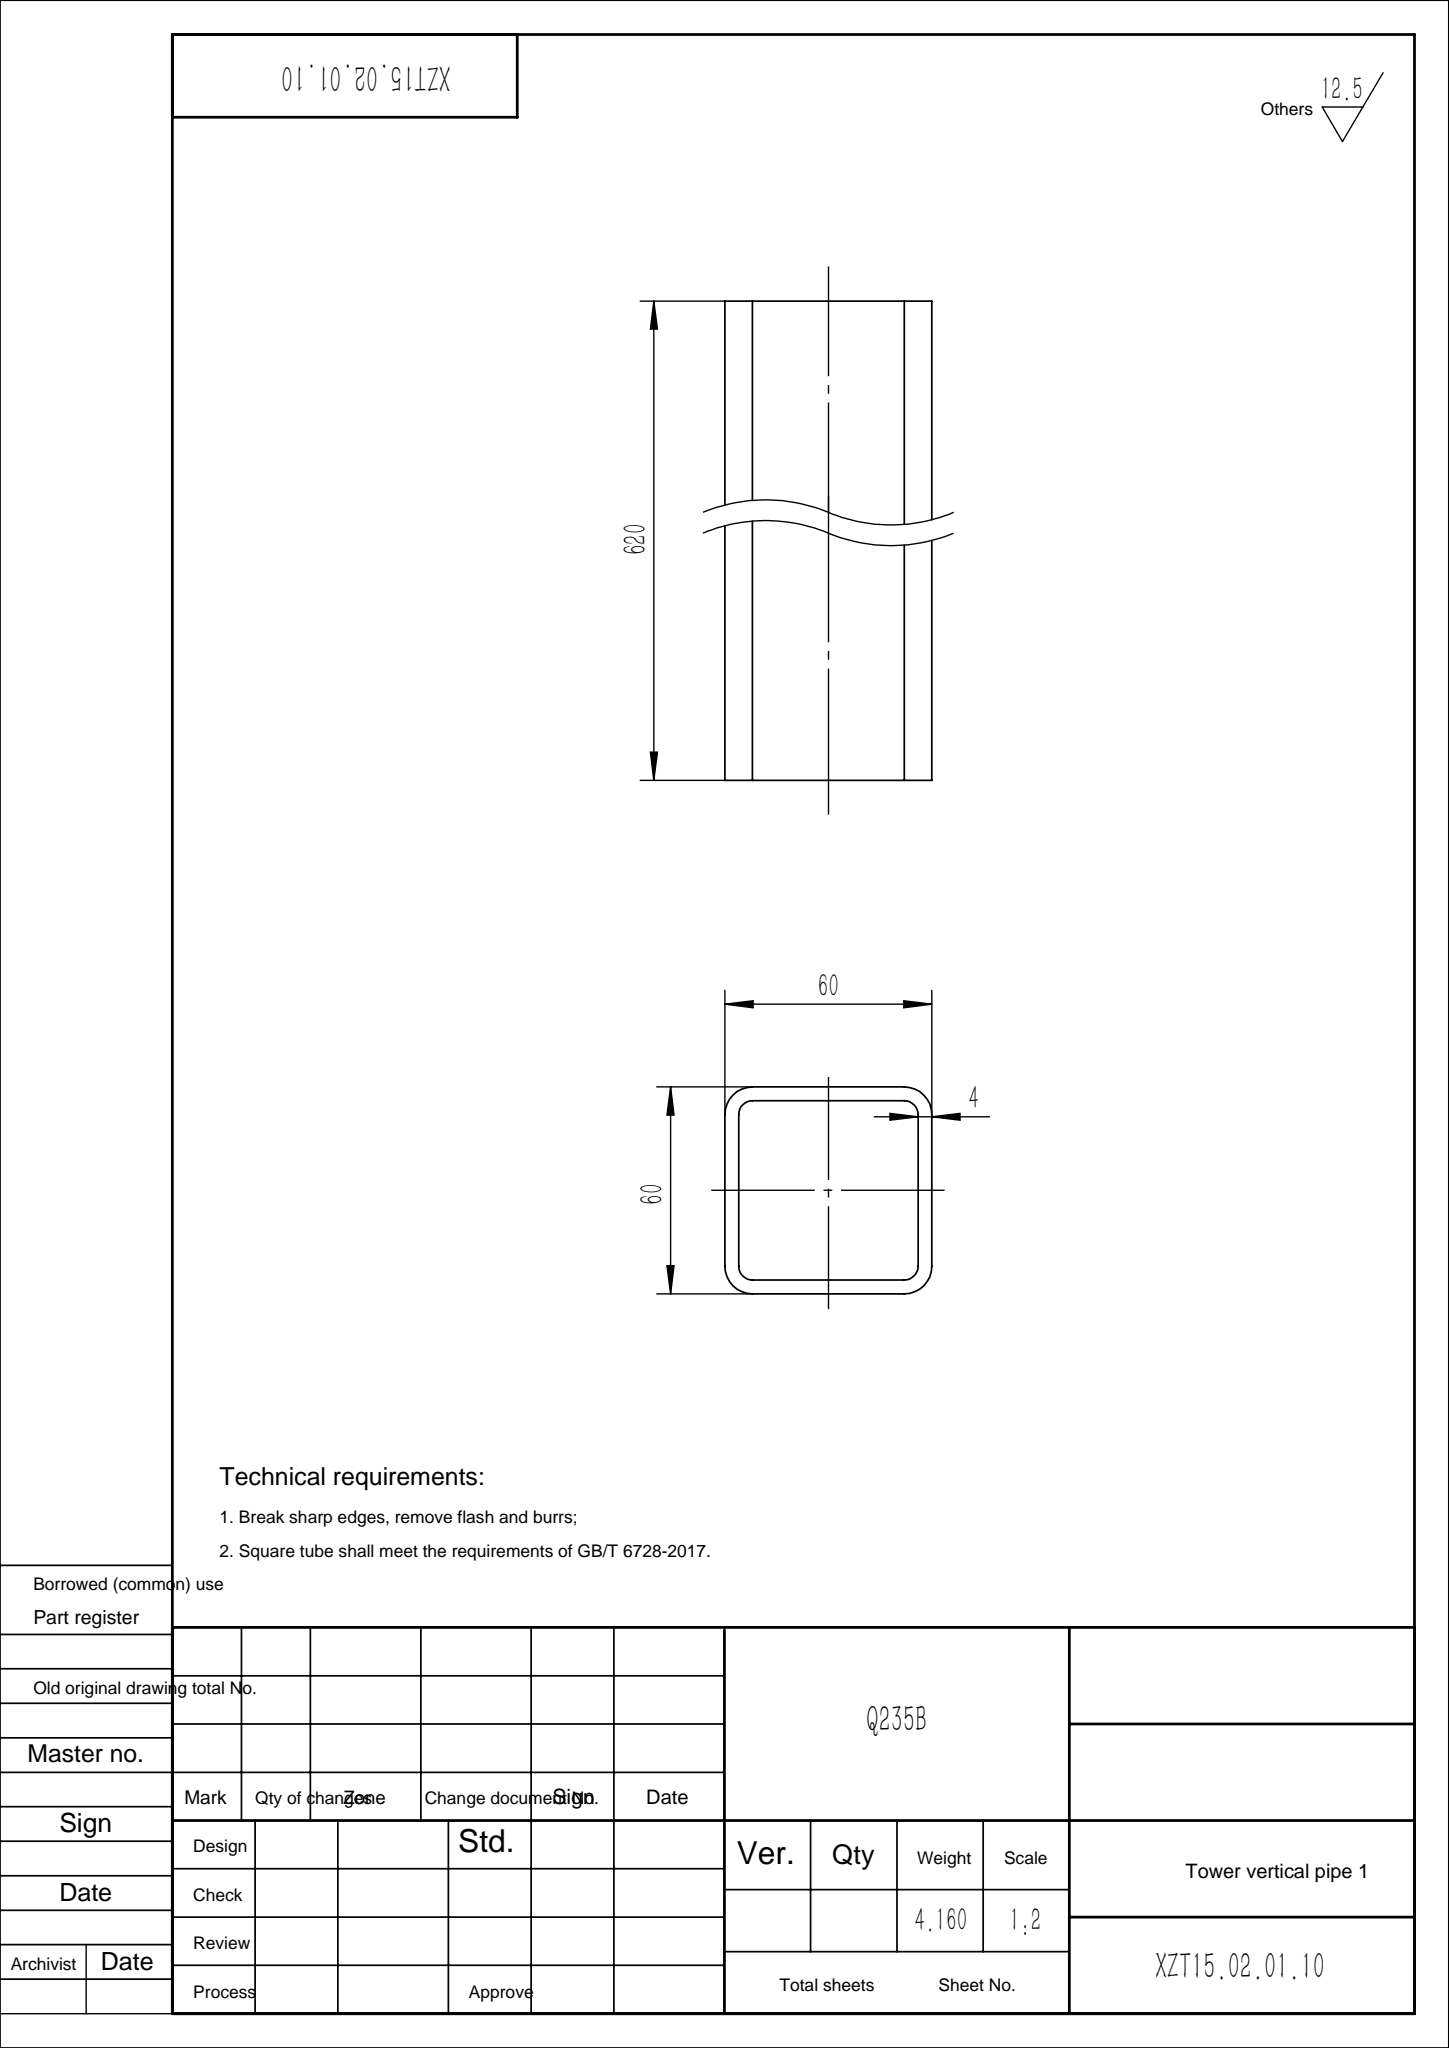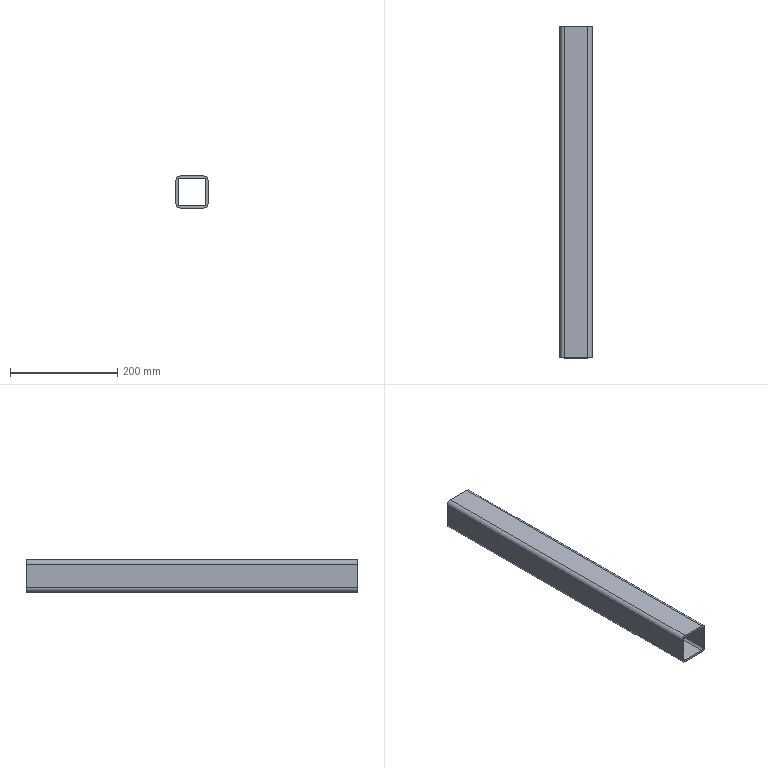Part | SolidWorks | features WeldMemberFeat 1, WeldmentFeature 1 | 1 solid | 18 faces | box 60 x 620 x 60 mm | volume 529974 mm3 | plane 10 | cylinder 8 | commonest cylinder face diameters 8 x4 16 x4
STEP:
#1=CARTESIAN_POINT('',(-30.,0.,22.));
#2=VERTEX_POINT('',#1);
#3=CARTESIAN_POINT('',(-22.,0.,30.));
#4=VERTEX_POINT('',#3);
#5=CARTESIAN_POINT('',(-22.,0.,22.));
#6=DIRECTION('',(0.,1.,0.));
#7=DIRECTION('',(0.,0.,1.));
#8=AXIS2_PLACEMENT_3D('',#5,#6,#7);
#9=CIRCLE('',#8,8.);
#10=EDGE_CURVE('',#2,#4,#9,.T.);
#11=ORIENTED_EDGE('',*,*,#10,.T.);
#12=CARTESIAN_POINT('',(-22.,620.,30.));
#13=VERTEX_POINT('',#12);
#14=CARTESIAN_POINT('',(-22.,620.,30.));
#15=DIRECTION('',(0.,-1.,0.));
#16=VECTOR('',#15,1000.);
#17=LINE('',#14,#16);
#18=EDGE_CURVE('',#13,#4,#17,.T.);
#19=ORIENTED_EDGE('',*,*,#18,.F.);
#20=CARTESIAN_POINT('',(-30.,620.,22.));
#21=VERTEX_POINT('',#20);
#22=CARTESIAN_POINT('',(-22.,620.,22.));
#23=DIRECTION('',(0.,1.,0.));
#24=DIRECTION('',(0.,0.,1.));
#25=AXIS2_PLACEMENT_3D('',#22,#23,#24);
#26=CIRCLE('',#25,8.);
#27=EDGE_CURVE('',#21,#13,#26,.T.);
#28=ORIENTED_EDGE('',*,*,#27,.F.);
#29=CARTESIAN_POINT('',(-30.,620.,22.));
#30=DIRECTION('',(0.,-1.,0.));
#31=VECTOR('',#30,1000.);
#32=LINE('',#29,#31);
#33=EDGE_CURVE('',#21,#2,#32,.T.);
#34=ORIENTED_EDGE('',*,*,#33,.T.);
#35=EDGE_LOOP('',(#11,#19,#28,#34));
#36=FACE_OUTER_BOUND('',#35,.T.);
#37=CARTESIAN_POINT('',(-22.,620.,22.));
#38=DIRECTION('',(0.,-1.,0.));
#39=DIRECTION('',(0.,0.,-1.));
#40=AXIS2_PLACEMENT_3D('',#37,#38,#39);
#41=CYLINDRICAL_SURFACE('',#40,8.);
#42=ADVANCED_FACE('',(#36),#41,.T.);
#43=CARTESIAN_POINT('',(22.,0.,30.));
#44=VERTEX_POINT('',#43);
#45=CARTESIAN_POINT('',(-22.,0.,30.));
#46=DIRECTION('',(1.,0.,0.));
#47=VECTOR('',#46,1000.);
#48=LINE('',#45,#47);
#49=EDGE_CURVE('',#4,#44,#48,.T.);
#50=ORIENTED_EDGE('',*,*,#49,.T.);
#51=CARTESIAN_POINT('',(22.,620.,30.));
#52=VERTEX_POINT('',#51);
#53=CARTESIAN_POINT('',(22.,620.,30.));
#54=DIRECTION('',(0.,-1.,0.));
#55=VECTOR('',#54,1000.);
#56=LINE('',#53,#55);
#57=EDGE_CURVE('',#52,#44,#56,.T.);
#58=ORIENTED_EDGE('',*,*,#57,.F.);
#59=CARTESIAN_POINT('',(-22.,620.,30.));
#60=DIRECTION('',(1.,0.,0.));
#61=VECTOR('',#60,1000.);
#62=LINE('',#59,#61);
#63=EDGE_CURVE('',#13,#52,#62,.T.);
#64=ORIENTED_EDGE('',*,*,#63,.F.);
#65=ORIENTED_EDGE('',*,*,#18,.T.);
#66=EDGE_LOOP('',(#50,#58,#64,#65));
#67=FACE_OUTER_BOUND('',#66,.T.);
#68=CARTESIAN_POINT('',(-22.,620.,30.));
#69=DIRECTION('',(0.,0.,-1.));
#70=DIRECTION('',(-1.,0.,0.));
#71=AXIS2_PLACEMENT_3D('',#68,#69,#70);
#72=PLANE('',#71);
#73=ADVANCED_FACE('',(#67),#72,.F.);
#74=CARTESIAN_POINT('',(30.,0.,22.));
#75=VERTEX_POINT('',#74);
#76=CARTESIAN_POINT('',(22.,0.,22.));
#77=DIRECTION('',(0.,1.,0.));
#78=DIRECTION('',(0.,0.,1.));
#79=AXIS2_PLACEMENT_3D('',#76,#77,#78);
#80=CIRCLE('',#79,8.);
#81=EDGE_CURVE('',#44,#75,#80,.T.);
#82=ORIENTED_EDGE('',*,*,#81,.T.);
#83=CARTESIAN_POINT('',(30.,620.,22.));
#84=VERTEX_POINT('',#83);
#85=CARTESIAN_POINT('',(30.,620.,22.));
#86=DIRECTION('',(0.,-1.,0.));
#87=VECTOR('',#86,1000.);
#88=LINE('',#85,#87);
#89=EDGE_CURVE('',#84,#75,#88,.T.);
#90=ORIENTED_EDGE('',*,*,#89,.F.);
#91=CARTESIAN_POINT('',(22.,620.,22.));
#92=DIRECTION('',(0.,1.,0.));
#93=DIRECTION('',(0.,0.,1.));
#94=AXIS2_PLACEMENT_3D('',#91,#92,#93);
#95=CIRCLE('',#94,8.);
#96=EDGE_CURVE('',#52,#84,#95,.T.);
#97=ORIENTED_EDGE('',*,*,#96,.F.);
#98=ORIENTED_EDGE('',*,*,#57,.T.);
#99=EDGE_LOOP('',(#82,#90,#97,#98));
#100=FACE_OUTER_BOUND('',#99,.T.);
#101=CARTESIAN_POINT('',(22.,620.,22.));
#102=DIRECTION('',(0.,-1.,0.));
#103=DIRECTION('',(0.,0.,-1.));
#104=AXIS2_PLACEMENT_3D('',#101,#102,#103);
#105=CYLINDRICAL_SURFACE('',#104,8.);
#106=ADVANCED_FACE('',(#100),#105,.T.);
#107=CARTESIAN_POINT('',(30.,0.,-22.));
#108=VERTEX_POINT('',#107);
#109=CARTESIAN_POINT('',(30.,0.,-22.));
#110=DIRECTION('',(0.,0.,-1.));
#111=VECTOR('',#110,1000.);
#112=LINE('',#109,#111);
#113=EDGE_CURVE('',#75,#108,#112,.T.);
#114=ORIENTED_EDGE('',*,*,#113,.T.);
#115=CARTESIAN_POINT('',(30.,620.,-22.));
#116=VERTEX_POINT('',#115);
#117=CARTESIAN_POINT('',(30.,620.,-22.));
#118=DIRECTION('',(0.,-1.,0.));
#119=VECTOR('',#118,1000.);
#120=LINE('',#117,#119);
#121=EDGE_CURVE('',#116,#108,#120,.T.);
#122=ORIENTED_EDGE('',*,*,#121,.F.);
#123=CARTESIAN_POINT('',(30.,620.,-22.));
#124=DIRECTION('',(0.,0.,-1.));
#125=VECTOR('',#124,1000.);
#126=LINE('',#123,#125);
#127=EDGE_CURVE('',#84,#116,#126,.T.);
#128=ORIENTED_EDGE('',*,*,#127,.F.);
#129=ORIENTED_EDGE('',*,*,#89,.T.);
#130=EDGE_LOOP('',(#114,#122,#128,#129));
#131=FACE_OUTER_BOUND('',#130,.T.);
#132=CARTESIAN_POINT('',(30.,620.,-22.));
#133=DIRECTION('',(-1.,0.,0.));
#134=DIRECTION('',(0.,0.,1.));
#135=AXIS2_PLACEMENT_3D('',#132,#133,#134);
#136=PLANE('',#135);
#137=ADVANCED_FACE('',(#131),#136,.F.);
#138=CARTESIAN_POINT('',(22.,0.,-30.));
#139=VERTEX_POINT('',#138);
#140=CARTESIAN_POINT('',(22.,0.,-22.));
#141=DIRECTION('',(0.,1.,0.));
#142=DIRECTION('',(0.,0.,1.));
#143=AXIS2_PLACEMENT_3D('',#140,#141,#142);
#144=CIRCLE('',#143,8.);
#145=EDGE_CURVE('',#108,#139,#144,.T.);
#146=ORIENTED_EDGE('',*,*,#145,.T.);
#147=CARTESIAN_POINT('',(22.,620.,-30.));
#148=VERTEX_POINT('',#147);
#149=CARTESIAN_POINT('',(22.,620.,-30.));
#150=DIRECTION('',(0.,-1.,0.));
#151=VECTOR('',#150,1000.);
#152=LINE('',#149,#151);
#153=EDGE_CURVE('',#148,#139,#152,.T.);
#154=ORIENTED_EDGE('',*,*,#153,.F.);
#155=CARTESIAN_POINT('',(22.,620.,-22.));
#156=DIRECTION('',(0.,1.,0.));
#157=DIRECTION('',(0.,0.,1.));
#158=AXIS2_PLACEMENT_3D('',#155,#156,#157);
#159=CIRCLE('',#158,8.);
#160=EDGE_CURVE('',#116,#148,#159,.T.);
#161=ORIENTED_EDGE('',*,*,#160,.F.);
#162=ORIENTED_EDGE('',*,*,#121,.T.);
#163=EDGE_LOOP('',(#146,#154,#161,#162));
#164=FACE_OUTER_BOUND('',#163,.T.);
#165=CARTESIAN_POINT('',(22.,620.,-22.));
#166=DIRECTION('',(0.,-1.,0.));
#167=DIRECTION('',(0.,0.,-1.));
#168=AXIS2_PLACEMENT_3D('',#165,#166,#167);
#169=CYLINDRICAL_SURFACE('',#168,8.);
#170=ADVANCED_FACE('',(#164),#169,.T.);
#171=CARTESIAN_POINT('',(-22.,0.,-30.));
#172=VERTEX_POINT('',#171);
#173=CARTESIAN_POINT('',(22.,0.,-30.));
#174=DIRECTION('',(-1.,0.,0.));
#175=VECTOR('',#174,1000.);
#176=LINE('',#173,#175);
#177=EDGE_CURVE('',#139,#172,#176,.T.);
#178=ORIENTED_EDGE('',*,*,#177,.T.);
#179=CARTESIAN_POINT('',(-22.,620.,-30.));
#180=VERTEX_POINT('',#179);
#181=CARTESIAN_POINT('',(-22.,620.,-30.));
#182=DIRECTION('',(0.,-1.,0.));
#183=VECTOR('',#182,1000.);
#184=LINE('',#181,#183);
#185=EDGE_CURVE('',#180,#172,#184,.T.);
#186=ORIENTED_EDGE('',*,*,#185,.F.);
#187=CARTESIAN_POINT('',(22.,620.,-30.));
#188=DIRECTION('',(-1.,0.,0.));
#189=VECTOR('',#188,1000.);
#190=LINE('',#187,#189);
#191=EDGE_CURVE('',#148,#180,#190,.T.);
#192=ORIENTED_EDGE('',*,*,#191,.F.);
#193=ORIENTED_EDGE('',*,*,#153,.T.);
#194=EDGE_LOOP('',(#178,#186,#192,#193));
#195=FACE_OUTER_BOUND('',#194,.T.);
#196=CARTESIAN_POINT('',(22.,620.,-30.));
#197=DIRECTION('',(0.,0.,1.));
#198=DIRECTION('',(1.,0.,0.));
#199=AXIS2_PLACEMENT_3D('',#196,#197,#198);
#200=PLANE('',#199);
#201=ADVANCED_FACE('',(#195),#200,.F.);
#202=CARTESIAN_POINT('',(-30.,0.,-22.));
#203=VERTEX_POINT('',#202);
#204=CARTESIAN_POINT('',(-22.,0.,-22.));
#205=DIRECTION('',(0.,1.,0.));
#206=DIRECTION('',(0.,0.,1.));
#207=AXIS2_PLACEMENT_3D('',#204,#205,#206);
#208=CIRCLE('',#207,8.);
#209=EDGE_CURVE('',#172,#203,#208,.T.);
#210=ORIENTED_EDGE('',*,*,#209,.T.);
#211=CARTESIAN_POINT('',(-30.,620.,-22.));
#212=VERTEX_POINT('',#211);
#213=CARTESIAN_POINT('',(-30.,620.,-22.));
#214=DIRECTION('',(0.,-1.,0.));
#215=VECTOR('',#214,1000.);
#216=LINE('',#213,#215);
#217=EDGE_CURVE('',#212,#203,#216,.T.);
#218=ORIENTED_EDGE('',*,*,#217,.F.);
#219=CARTESIAN_POINT('',(-22.,620.,-22.));
#220=DIRECTION('',(0.,1.,0.));
#221=DIRECTION('',(0.,0.,1.));
#222=AXIS2_PLACEMENT_3D('',#219,#220,#221);
#223=CIRCLE('',#222,8.);
#224=EDGE_CURVE('',#180,#212,#223,.T.);
#225=ORIENTED_EDGE('',*,*,#224,.F.);
#226=ORIENTED_EDGE('',*,*,#185,.T.);
#227=EDGE_LOOP('',(#210,#218,#225,#226));
#228=FACE_OUTER_BOUND('',#227,.T.);
#229=CARTESIAN_POINT('',(-22.,620.,-22.));
#230=DIRECTION('',(0.,-1.,0.));
#231=DIRECTION('',(0.,0.,-1.));
#232=AXIS2_PLACEMENT_3D('',#229,#230,#231);
#233=CYLINDRICAL_SURFACE('',#232,8.);
#234=ADVANCED_FACE('',(#228),#233,.T.);
#235=CARTESIAN_POINT('',(22.,0.,26.));
#236=VERTEX_POINT('',#235);
#237=CARTESIAN_POINT('',(26.,0.,22.));
#238=VERTEX_POINT('',#237);
#239=CARTESIAN_POINT('',(22.,0.,22.));
#240=DIRECTION('',(0.,1.,0.));
#241=DIRECTION('',(0.,0.,1.));
#242=AXIS2_PLACEMENT_3D('',#239,#240,#241);
#243=CIRCLE('',#242,4.);
#244=EDGE_CURVE('',#236,#238,#243,.T.);
#245=ORIENTED_EDGE('',*,*,#244,.F.);
#246=CARTESIAN_POINT('',(22.,620.,26.));
#247=VERTEX_POINT('',#246);
#248=CARTESIAN_POINT('',(22.,620.,26.));
#249=DIRECTION('',(0.,-1.,0.));
#250=VECTOR('',#249,1000.);
#251=LINE('',#248,#250);
#252=EDGE_CURVE('',#247,#236,#251,.T.);
#253=ORIENTED_EDGE('',*,*,#252,.F.);
#254=CARTESIAN_POINT('',(26.,620.,22.));
#255=VERTEX_POINT('',#254);
#256=CARTESIAN_POINT('',(22.,620.,22.));
#257=DIRECTION('',(0.,1.,0.));
#258=DIRECTION('',(0.,0.,1.));
#259=AXIS2_PLACEMENT_3D('',#256,#257,#258);
#260=CIRCLE('',#259,4.);
#261=EDGE_CURVE('',#247,#255,#260,.T.);
#262=ORIENTED_EDGE('',*,*,#261,.T.);
#263=CARTESIAN_POINT('',(26.,620.,22.));
#264=DIRECTION('',(0.,-1.,0.));
#265=VECTOR('',#264,1000.);
#266=LINE('',#263,#265);
#267=EDGE_CURVE('',#255,#238,#266,.T.);
#268=ORIENTED_EDGE('',*,*,#267,.T.);
#269=EDGE_LOOP('',(#245,#253,#262,#268));
#270=FACE_OUTER_BOUND('',#269,.T.);
#271=CARTESIAN_POINT('',(22.,620.,22.));
#272=DIRECTION('',(0.,-1.,0.));
#273=DIRECTION('',(0.,0.,-1.));
#274=AXIS2_PLACEMENT_3D('',#271,#272,#273);
#275=CYLINDRICAL_SURFACE('',#274,4.);
#276=ADVANCED_FACE('',(#270),#275,.F.);
#277=CARTESIAN_POINT('',(-22.,0.,26.));
#278=VERTEX_POINT('',#277);
#279=CARTESIAN_POINT('',(-22.,0.,26.));
#280=DIRECTION('',(1.,0.,0.));
#281=VECTOR('',#280,1000.);
#282=LINE('',#279,#281);
#283=EDGE_CURVE('',#278,#236,#282,.T.);
#284=ORIENTED_EDGE('',*,*,#283,.F.);
#285=CARTESIAN_POINT('',(-22.,620.,26.));
#286=VERTEX_POINT('',#285);
#287=CARTESIAN_POINT('',(-22.,620.,26.));
#288=DIRECTION('',(0.,-1.,0.));
#289=VECTOR('',#288,1000.);
#290=LINE('',#287,#289);
#291=EDGE_CURVE('',#286,#278,#290,.T.);
#292=ORIENTED_EDGE('',*,*,#291,.F.);
#293=CARTESIAN_POINT('',(-22.,620.,26.));
#294=DIRECTION('',(1.,0.,0.));
#295=VECTOR('',#294,1000.);
#296=LINE('',#293,#295);
#297=EDGE_CURVE('',#286,#247,#296,.T.);
#298=ORIENTED_EDGE('',*,*,#297,.T.);
#299=ORIENTED_EDGE('',*,*,#252,.T.);
#300=EDGE_LOOP('',(#284,#292,#298,#299));
#301=FACE_OUTER_BOUND('',#300,.T.);
#302=CARTESIAN_POINT('',(-22.,620.,26.));
#303=DIRECTION('',(0.,0.,-1.));
#304=DIRECTION('',(-1.,0.,0.));
#305=AXIS2_PLACEMENT_3D('',#302,#303,#304);
#306=PLANE('',#305);
#307=ADVANCED_FACE('',(#301),#306,.T.);
#308=CARTESIAN_POINT('',(-26.,0.,22.));
#309=VERTEX_POINT('',#308);
#310=CARTESIAN_POINT('',(-22.,0.,22.));
#311=DIRECTION('',(0.,1.,0.));
#312=DIRECTION('',(0.,0.,1.));
#313=AXIS2_PLACEMENT_3D('',#310,#311,#312);
#314=CIRCLE('',#313,4.);
#315=EDGE_CURVE('',#309,#278,#314,.T.);
#316=ORIENTED_EDGE('',*,*,#315,.F.);
#317=CARTESIAN_POINT('',(-26.,620.,22.));
#318=VERTEX_POINT('',#317);
#319=CARTESIAN_POINT('',(-26.,620.,22.));
#320=DIRECTION('',(0.,-1.,0.));
#321=VECTOR('',#320,1000.);
#322=LINE('',#319,#321);
#323=EDGE_CURVE('',#318,#309,#322,.T.);
#324=ORIENTED_EDGE('',*,*,#323,.F.);
#325=CARTESIAN_POINT('',(-22.,620.,22.));
#326=DIRECTION('',(0.,1.,0.));
#327=DIRECTION('',(0.,0.,1.));
#328=AXIS2_PLACEMENT_3D('',#325,#326,#327);
#329=CIRCLE('',#328,4.);
#330=EDGE_CURVE('',#318,#286,#329,.T.);
#331=ORIENTED_EDGE('',*,*,#330,.T.);
#332=ORIENTED_EDGE('',*,*,#291,.T.);
#333=EDGE_LOOP('',(#316,#324,#331,#332));
#334=FACE_OUTER_BOUND('',#333,.T.);
#335=CARTESIAN_POINT('',(-22.,620.,22.));
#336=DIRECTION('',(0.,-1.,0.));
#337=DIRECTION('',(0.,0.,-1.));
#338=AXIS2_PLACEMENT_3D('',#335,#336,#337);
#339=CYLINDRICAL_SURFACE('',#338,4.);
#340=ADVANCED_FACE('',(#334),#339,.F.);
#341=CARTESIAN_POINT('',(-26.,0.,-22.));
#342=VERTEX_POINT('',#341);
#343=CARTESIAN_POINT('',(-26.,0.,22.));
#344=DIRECTION('',(0.,0.,1.));
#345=VECTOR('',#344,1000.);
#346=LINE('',#343,#345);
#347=EDGE_CURVE('',#342,#309,#346,.T.);
#348=ORIENTED_EDGE('',*,*,#347,.F.);
#349=CARTESIAN_POINT('',(-26.,620.,-22.));
#350=VERTEX_POINT('',#349);
#351=CARTESIAN_POINT('',(-26.,620.,-22.));
#352=DIRECTION('',(0.,-1.,0.));
#353=VECTOR('',#352,1000.);
#354=LINE('',#351,#353);
#355=EDGE_CURVE('',#350,#342,#354,.T.);
#356=ORIENTED_EDGE('',*,*,#355,.F.);
#357=CARTESIAN_POINT('',(-26.,620.,22.));
#358=DIRECTION('',(0.,0.,1.));
#359=VECTOR('',#358,1000.);
#360=LINE('',#357,#359);
#361=EDGE_CURVE('',#350,#318,#360,.T.);
#362=ORIENTED_EDGE('',*,*,#361,.T.);
#363=ORIENTED_EDGE('',*,*,#323,.T.);
#364=EDGE_LOOP('',(#348,#356,#362,#363));
#365=FACE_OUTER_BOUND('',#364,.T.);
#366=CARTESIAN_POINT('',(-26.,620.,22.));
#367=DIRECTION('',(1.,0.,0.));
#368=DIRECTION('',(0.,0.,-1.));
#369=AXIS2_PLACEMENT_3D('',#366,#367,#368);
#370=PLANE('',#369);
#371=ADVANCED_FACE('',(#365),#370,.T.);
#372=CARTESIAN_POINT('',(-22.,0.,-26.));
#373=VERTEX_POINT('',#372);
#374=CARTESIAN_POINT('',(-22.,0.,-22.));
#375=DIRECTION('',(0.,1.,0.));
#376=DIRECTION('',(0.,0.,1.));
#377=AXIS2_PLACEMENT_3D('',#374,#375,#376);
#378=CIRCLE('',#377,4.);
#379=EDGE_CURVE('',#373,#342,#378,.T.);
#380=ORIENTED_EDGE('',*,*,#379,.F.);
#381=CARTESIAN_POINT('',(-22.,620.,-26.));
#382=VERTEX_POINT('',#381);
#383=CARTESIAN_POINT('',(-22.,620.,-26.));
#384=DIRECTION('',(0.,-1.,0.));
#385=VECTOR('',#384,1000.);
#386=LINE('',#383,#385);
#387=EDGE_CURVE('',#382,#373,#386,.T.);
#388=ORIENTED_EDGE('',*,*,#387,.F.);
#389=CARTESIAN_POINT('',(-22.,620.,-22.));
#390=DIRECTION('',(0.,1.,0.));
#391=DIRECTION('',(0.,0.,1.));
#392=AXIS2_PLACEMENT_3D('',#389,#390,#391);
#393=CIRCLE('',#392,4.);
#394=EDGE_CURVE('',#382,#350,#393,.T.);
#395=ORIENTED_EDGE('',*,*,#394,.T.);
#396=ORIENTED_EDGE('',*,*,#355,.T.);
#397=EDGE_LOOP('',(#380,#388,#395,#396));
#398=FACE_OUTER_BOUND('',#397,.T.);
#399=CARTESIAN_POINT('',(-22.,620.,-22.));
#400=DIRECTION('',(0.,-1.,0.));
#401=DIRECTION('',(0.,0.,-1.));
#402=AXIS2_PLACEMENT_3D('',#399,#400,#401);
#403=CYLINDRICAL_SURFACE('',#402,4.);
#404=ADVANCED_FACE('',(#398),#403,.F.);
#405=CARTESIAN_POINT('',(22.,0.,-26.));
#406=VERTEX_POINT('',#405);
#407=CARTESIAN_POINT('',(22.,0.,-26.));
#408=DIRECTION('',(-1.,0.,0.));
#409=VECTOR('',#408,1000.);
#410=LINE('',#407,#409);
#411=EDGE_CURVE('',#406,#373,#410,.T.);
#412=ORIENTED_EDGE('',*,*,#411,.F.);
#413=CARTESIAN_POINT('',(22.,620.,-26.));
#414=VERTEX_POINT('',#413);
#415=CARTESIAN_POINT('',(22.,620.,-26.));
#416=DIRECTION('',(0.,-1.,0.));
#417=VECTOR('',#416,1000.);
#418=LINE('',#415,#417);
#419=EDGE_CURVE('',#414,#406,#418,.T.);
#420=ORIENTED_EDGE('',*,*,#419,.F.);
#421=CARTESIAN_POINT('',(22.,620.,-26.));
#422=DIRECTION('',(-1.,0.,0.));
#423=VECTOR('',#422,1000.);
#424=LINE('',#421,#423);
#425=EDGE_CURVE('',#414,#382,#424,.T.);
#426=ORIENTED_EDGE('',*,*,#425,.T.);
#427=ORIENTED_EDGE('',*,*,#387,.T.);
#428=EDGE_LOOP('',(#412,#420,#426,#427));
#429=FACE_OUTER_BOUND('',#428,.T.);
#430=CARTESIAN_POINT('',(22.,620.,-26.));
#431=DIRECTION('',(0.,0.,1.));
#432=DIRECTION('',(1.,0.,0.));
#433=AXIS2_PLACEMENT_3D('',#430,#431,#432);
#434=PLANE('',#433);
#435=ADVANCED_FACE('',(#429),#434,.T.);
#436=CARTESIAN_POINT('',(26.,0.,-22.));
#437=VERTEX_POINT('',#436);
#438=CARTESIAN_POINT('',(22.,0.,-22.));
#439=DIRECTION('',(0.,1.,0.));
#440=DIRECTION('',(0.,0.,1.));
#441=AXIS2_PLACEMENT_3D('',#438,#439,#440);
#442=CIRCLE('',#441,4.);
#443=EDGE_CURVE('',#437,#406,#442,.T.);
#444=ORIENTED_EDGE('',*,*,#443,.F.);
#445=CARTESIAN_POINT('',(26.,620.,-22.));
#446=VERTEX_POINT('',#445);
#447=CARTESIAN_POINT('',(26.,620.,-22.));
#448=DIRECTION('',(0.,-1.,0.));
#449=VECTOR('',#448,1000.);
#450=LINE('',#447,#449);
#451=EDGE_CURVE('',#446,#437,#450,.T.);
#452=ORIENTED_EDGE('',*,*,#451,.F.);
#453=CARTESIAN_POINT('',(22.,620.,-22.));
#454=DIRECTION('',(0.,1.,0.));
#455=DIRECTION('',(0.,0.,1.));
#456=AXIS2_PLACEMENT_3D('',#453,#454,#455);
#457=CIRCLE('',#456,4.);
#458=EDGE_CURVE('',#446,#414,#457,.T.);
#459=ORIENTED_EDGE('',*,*,#458,.T.);
#460=ORIENTED_EDGE('',*,*,#419,.T.);
#461=EDGE_LOOP('',(#444,#452,#459,#460));
#462=FACE_OUTER_BOUND('',#461,.T.);
#463=CARTESIAN_POINT('',(22.,620.,-22.));
#464=DIRECTION('',(0.,-1.,0.));
#465=DIRECTION('',(0.,0.,-1.));
#466=AXIS2_PLACEMENT_3D('',#463,#464,#465);
#467=CYLINDRICAL_SURFACE('',#466,4.);
#468=ADVANCED_FACE('',(#462),#467,.F.);
#469=CARTESIAN_POINT('',(26.,0.,-22.));
#470=DIRECTION('',(0.,0.,-1.));
#471=VECTOR('',#470,1000.);
#472=LINE('',#469,#471);
#473=EDGE_CURVE('',#238,#437,#472,.T.);
#474=ORIENTED_EDGE('',*,*,#473,.F.);
#475=ORIENTED_EDGE('',*,*,#267,.F.);
#476=CARTESIAN_POINT('',(26.,620.,-22.));
#477=DIRECTION('',(0.,0.,-1.));
#478=VECTOR('',#477,1000.);
#479=LINE('',#476,#478);
#480=EDGE_CURVE('',#255,#446,#479,.T.);
#481=ORIENTED_EDGE('',*,*,#480,.T.);
#482=ORIENTED_EDGE('',*,*,#451,.T.);
#483=EDGE_LOOP('',(#474,#475,#481,#482));
#484=FACE_OUTER_BOUND('',#483,.T.);
#485=CARTESIAN_POINT('',(26.,620.,-22.));
#486=DIRECTION('',(-1.,0.,0.));
#487=DIRECTION('',(0.,0.,1.));
#488=AXIS2_PLACEMENT_3D('',#485,#486,#487);
#489=PLANE('',#488);
#490=ADVANCED_FACE('',(#484),#489,.T.);
#491=CARTESIAN_POINT('',(-30.,0.,22.));
#492=DIRECTION('',(0.,0.,1.));
#493=VECTOR('',#492,1000.);
#494=LINE('',#491,#493);
#495=EDGE_CURVE('',#203,#2,#494,.T.);
#496=ORIENTED_EDGE('',*,*,#495,.T.);
#497=ORIENTED_EDGE('',*,*,#33,.F.);
#498=CARTESIAN_POINT('',(-30.,620.,22.));
#499=DIRECTION('',(0.,0.,1.));
#500=VECTOR('',#499,1000.);
#501=LINE('',#498,#500);
#502=EDGE_CURVE('',#212,#21,#501,.T.);
#503=ORIENTED_EDGE('',*,*,#502,.F.);
#504=ORIENTED_EDGE('',*,*,#217,.T.);
#505=EDGE_LOOP('',(#496,#497,#503,#504));
#506=FACE_OUTER_BOUND('',#505,.T.);
#507=CARTESIAN_POINT('',(-30.,620.,22.));
#508=DIRECTION('',(1.,0.,0.));
#509=DIRECTION('',(0.,0.,-1.));
#510=AXIS2_PLACEMENT_3D('',#507,#508,#509);
#511=PLANE('',#510);
#512=ADVANCED_FACE('',(#506),#511,.F.);
#513=ORIENTED_EDGE('',*,*,#261,.F.);
#514=ORIENTED_EDGE('',*,*,#297,.F.);
#515=ORIENTED_EDGE('',*,*,#330,.F.);
#516=ORIENTED_EDGE('',*,*,#361,.F.);
#517=ORIENTED_EDGE('',*,*,#394,.F.);
#518=ORIENTED_EDGE('',*,*,#425,.F.);
#519=ORIENTED_EDGE('',*,*,#458,.F.);
#520=ORIENTED_EDGE('',*,*,#480,.F.);
#521=EDGE_LOOP('',(#513,#514,#515,#516,#517,#518,#519,#520));
#522=FACE_BOUND('',#521,.T.);
#523=ORIENTED_EDGE('',*,*,#27,.T.);
#524=ORIENTED_EDGE('',*,*,#63,.T.);
#525=ORIENTED_EDGE('',*,*,#96,.T.);
#526=ORIENTED_EDGE('',*,*,#127,.T.);
#527=ORIENTED_EDGE('',*,*,#160,.T.);
#528=ORIENTED_EDGE('',*,*,#191,.T.);
#529=ORIENTED_EDGE('',*,*,#224,.T.);
#530=ORIENTED_EDGE('',*,*,#502,.T.);
#531=EDGE_LOOP('',(#523,#524,#525,#526,#527,#528,#529,#530));
#532=FACE_OUTER_BOUND('',#531,.T.);
#533=CARTESIAN_POINT('',(-22.,620.,22.));
#534=DIRECTION('',(0.,1.,0.));
#535=DIRECTION('',(0.,0.,1.));
#536=AXIS2_PLACEMENT_3D('',#533,#534,#535);
#537=PLANE('',#536);
#538=ADVANCED_FACE('',(#522,#532),#537,.T.);
#539=ORIENTED_EDGE('',*,*,#244,.T.);
#540=ORIENTED_EDGE('',*,*,#473,.T.);
#541=ORIENTED_EDGE('',*,*,#443,.T.);
#542=ORIENTED_EDGE('',*,*,#411,.T.);
#543=ORIENTED_EDGE('',*,*,#379,.T.);
#544=ORIENTED_EDGE('',*,*,#347,.T.);
#545=ORIENTED_EDGE('',*,*,#315,.T.);
#546=ORIENTED_EDGE('',*,*,#283,.T.);
#547=EDGE_LOOP('',(#539,#540,#541,#542,#543,#544,#545,#546));
#548=FACE_BOUND('',#547,.T.);
#549=ORIENTED_EDGE('',*,*,#10,.F.);
#550=ORIENTED_EDGE('',*,*,#495,.F.);
#551=ORIENTED_EDGE('',*,*,#209,.F.);
#552=ORIENTED_EDGE('',*,*,#177,.F.);
#553=ORIENTED_EDGE('',*,*,#145,.F.);
#554=ORIENTED_EDGE('',*,*,#113,.F.);
#555=ORIENTED_EDGE('',*,*,#81,.F.);
#556=ORIENTED_EDGE('',*,*,#49,.F.);
#557=EDGE_LOOP('',(#549,#550,#551,#552,#553,#554,#555,#556));
#558=FACE_OUTER_BOUND('',#557,.T.);
#559=CARTESIAN_POINT('',(-22.,0.,22.));
#560=DIRECTION('',(0.,1.,0.));
#561=DIRECTION('',(0.,0.,1.));
#562=AXIS2_PLACEMENT_3D('',#559,#560,#561);
#563=PLANE('',#562);
#564=ADVANCED_FACE('',(#548,#558),#563,.F.);
#565=CLOSED_SHELL('',(#42,#73,#106,#137,#170,#201,#234,#276,#307,#340,#371,#404,#435,#468,#490,#512,#538,#564));
#566=MANIFOLD_SOLID_BREP('',#565);
#567=CARTESIAN_POINT('',(0.,0.,0.));
#568=DIRECTION('',(0.,0.,1.));
#569=DIRECTION('',(1.,0.,0.));
#570=AXIS2_PLACEMENT_3D('',#567,#568,#569);
#571=(LENGTH_UNIT()NAMED_UNIT(*)SI_UNIT(.MILLI.,.METRE.));
#572=UNCERTAINTY_MEASURE_WITH_UNIT(LENGTH_MEASURE(0.00001),#571,'','');
#573=(NAMED_UNIT(*)PLANE_ANGLE_UNIT()SI_UNIT($,.RADIAN.));
#574=(NAMED_UNIT(*)SI_UNIT($,.STERADIAN.)SOLID_ANGLE_UNIT());
#575=(GEOMETRIC_REPRESENTATION_CONTEXT(3)GLOBAL_UNCERTAINTY_ASSIGNED_CONTEXT((#572))GLOBAL_UNIT_ASSIGNED_CONTEXT((#571,#573,#574))REPRESENTATION_CONTEXT('',''));
#576=ADVANCED_BREP_SHAPE_REPRESENTATION('',(#566,#570),#575);